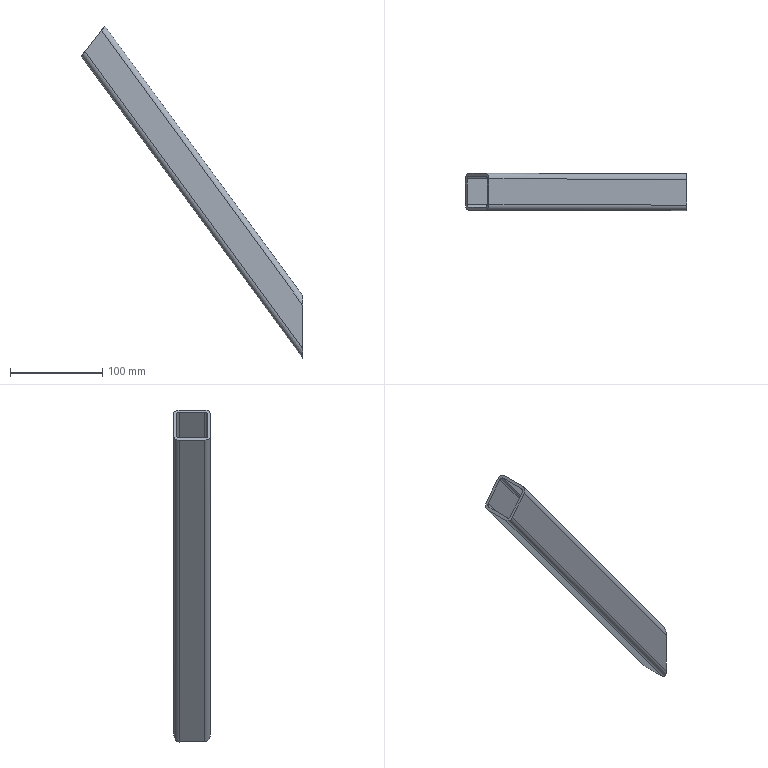Part | STEP file | front baffle frame | 1 solid | 18 faces | box 240.241 x 40 x 360.346 mm | volume 161857 mm3 | plane 10 | cylinder 8 | commonest cylinder face diameters 6 x4 12 x4